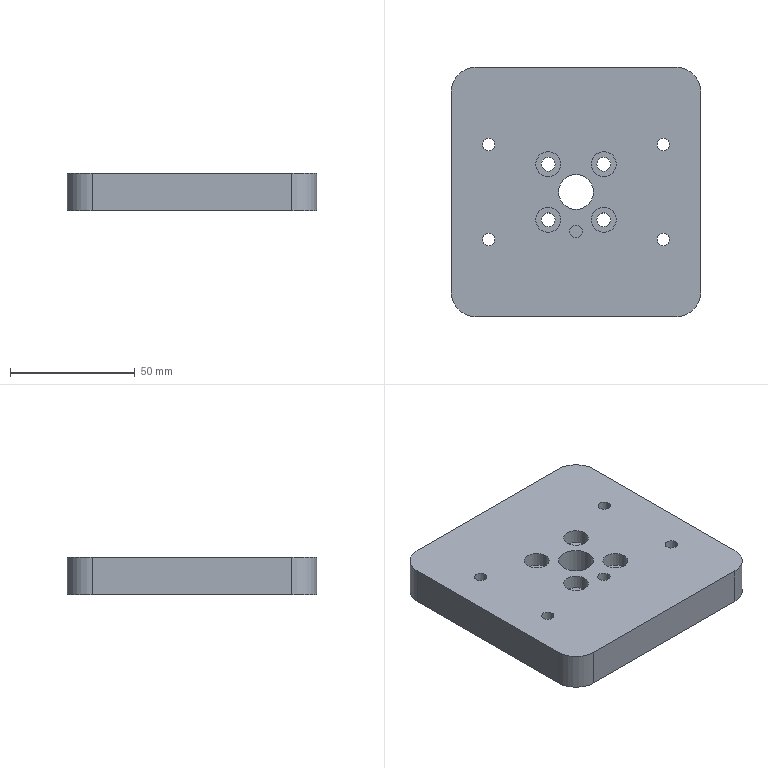NC program | NX | posted with a generic post | part box 100 x 100 x 15 mm
Lines 25 to 851 of 2072:
(ZLEVEL_PROFILE , TOOL : D10)
N48 T10 M6
N50 G54
N52 G17 G0 G90 X-53.748 Y-46.229 S9500 M3
N54 G43 Z30. H10
N56 Z1.5
N58 G94 G1 X-54.028 Y-45.669 Z1.467 F1000.
N60 X-54.754 Y-43.354 Z1.34
N62 X-55.1 Y-40.952 Z1.213
N64 Y-40. Z1.163
N66 Y0. Z-0.933
N68 Y40. F3500.
N70 G2 X-40. Y55.1 R15.1
N72 G1 X40.
N74 G2 X55.1 Y40. R15.1
N76 G1 Y-40.
N78 G2 X40. Y-55.1 R15.1
N80 G1 X-40.
N82 G2 X-55.1 Y-40. R15.1
N84 G1 Y0.
N86 Y40. Z-1.023
N88 X-55.072 Y40.912 Z-1.025
N90 X-54.99 Y41.82 Z-1.027
N92 X-54.853 Y42.722 Z-1.029
N94 X-54.661 Y43.614 Z-1.032
N96 X-54.416 Y44.492 Z-1.034
N98 X-54.119 Y45.355 Z-1.036
N100 X-53.77 Y46.197 Z-1.038
N102 X-53.37 Y47.017 Z-1.04
N104 X-52.922 Y47.812 Z-1.042
N106 X-52.427 Y48.578 Z-1.044
N108 X-51.886 Y49.312 Z-1.046
N110 X-51.303 Y50.013 Z-1.048
N112 X-50.677 Y50.677 Z-1.05
N114 X-50.013 Y51.303 Z-1.052
N116 X-49.312 Y51.886 Z-1.054
N118 X-48.578 Y52.427 Z-1.056
N120 X-47.812 Y52.922 Z-1.058
N122 X-47.017 Y53.37 Z-1.06
N124 X-46.197 Y53.77 Z-1.062
N126 X-45.355 Y54.119 Z-1.064
N128 X-44.492 Y54.416 Z-1.066
N130 X-43.614 Y54.661 Z-1.068
N132 X-42.722 Y54.853 Z-1.071
N134 X-41.82 Y54.99 Z-1.073
N136 X-40.912 Y55.072 Z-1.075
N138 X-40. Y55.1 Z-1.077
N140 X40. Z-1.257
N142 X40.912 Y55.072 Z-1.259
N144 X41.82 Y54.99 Z-1.261
N146 X42.722 Y54.853 Z-1.263
N148 X43.614 Y54.661 Z-1.265
N150 X44.492 Y54.416 Z-1.267
N152 X45.355 Y54.119 Z-1.269
N154 X46.197 Y53.77 Z-1.271
N156 X47.017 Y53.37 Z-1.273
N158 X47.812 Y52.922 Z-1.275
N160 X48.578 Y52.427 Z-1.277
N162 X49.312 Y51.886 Z-1.279
N164 X50.013 Y51.303 Z-1.281
N166 X50.677 Y50.677 Z-1.283
N168 X51.303 Y50.013 Z-1.285
N170 X51.886 Y49.312 Z-1.287
N172 X52.427 Y48.578 Z-1.289
N174 X52.922 Y47.812 Z-1.292
N176 X53.37 Y47.017 Z-1.294
N178 X53.77 Y46.197 Z-1.296
N180 X54.119 Y45.355 Z-1.298
N182 X54.416 Y44.492 Z-1.3
N184 X54.661 Y43.614 Z-1.302
N186 X54.853 Y42.722 Z-1.304
N188 X54.99 Y41.82 Z-1.306
N190 X55.072 Y40.912 Z-1.308
N192 X55.1 Y40. Z-1.31
N194 Y-40. Z-1.49
N196 X55.072 Y-40.912 Z-1.492
N198 X54.99 Y-41.82 Z-1.494
N200 X54.853 Y-42.722 Z-1.496
N202 X54.661 Y-43.614 Z-1.498
N204 X54.416 Y-44.492 Z-1.5
N206 X54.119 Y-45.355 Z-1.502
N208 X53.77 Y-46.197 Z-1.504
N210 X53.37 Y-47.017 Z-1.506
N212 X52.922 Y-47.812 Z-1.508
N214 X52.427 Y-48.578 Z-1.511
N216 X51.886 Y-49.312 Z-1.513
N218 X51.303 Y-50.013 Z-1.515
N220 X50.677 Y-50.677 Z-1.517
N222 X50.013 Y-51.303 Z-1.519
N224 X49.312 Y-51.886 Z-1.521
N226 X48.578 Y-52.427 Z-1.523
N228 X47.812 Y-52.922 Z-1.525
N230 X47.017 Y-53.37 Z-1.527
N232 X46.197 Y-53.77 Z-1.529
N234 X45.355 Y-54.119 Z-1.531
N236 X44.492 Y-54.416 Z-1.533
N238 X43.614 Y-54.661 Z-1.535
N240 X42.722 Y-54.853 Z-1.537
N242 X41.82 Y-54.99 Z-1.539
N244 X40.912 Y-55.072 Z-1.541
N246 X40. Y-55.1 Z-1.543
N248 X-40. Z-1.723
N250 X-40.912 Y-55.072 Z-1.725
N252 X-41.82 Y-54.99 Z-1.727
N254 X-42.722 Y-54.853 Z-1.729
N256 X-43.614 Y-54.661 Z-1.732
N258 X-44.492 Y-54.416 Z-1.734
N260 X-45.355 Y-54.119 Z-1.736
N262 X-46.197 Y-53.77 Z-1.738
N264 X-47.017 Y-53.37 Z-1.74
N266 X-47.812 Y-52.922 Z-1.742
N268 X-48.578 Y-52.427 Z-1.744
N270 X-49.312 Y-51.886 Z-1.746
N272 X-50.013 Y-51.303 Z-1.748
N274 X-50.677 Y-50.677 Z-1.75
N276 X-51.303 Y-50.013 Z-1.752
N278 X-51.886 Y-49.312 Z-1.754
N280 X-52.427 Y-48.578 Z-1.756
N282 X-52.922 Y-47.812 Z-1.758
N284 X-53.37 Y-47.017 Z-1.76
N286 X-53.77 Y-46.197 Z-1.762
N288 X-54.119 Y-45.355 Z-1.764
N290 X-54.416 Y-44.492 Z-1.766
N292 X-54.661 Y-43.614 Z-1.768
N294 X-54.853 Y-42.722 Z-1.771
N296 X-54.99 Y-41.82 Z-1.773
N298 X-55.072 Y-40.912 Z-1.775
N300 X-55.1 Y-40. Z-1.777
N302 Y0. Z-1.867
N304 Y40. Z-1.957
N306 X-55.072 Y40.912 Z-1.959
N308 X-54.99 Y41.82 Z-1.961
N310 X-54.853 Y42.722 Z-1.963
N312 X-54.661 Y43.614 Z-1.965
N314 X-54.416 Y44.492 Z-1.967
N316 X-54.119 Y45.355 Z-1.969
N318 X-53.77 Y46.197 Z-1.971
N320 X-53.37 Y47.017 Z-1.973
N322 X-52.922 Y47.812 Z-1.975
N324 X-52.427 Y48.578 Z-1.977
N326 X-51.886 Y49.312 Z-1.979
N328 X-51.303 Y50.013 Z-1.981
N330 X-50.677 Y50.677 Z-1.983
N332 X-50.013 Y51.303 Z-1.985
N334 X-49.312 Y51.886 Z-1.987
N336 X-48.578 Y52.427 Z-1.989
N338 X-47.812 Y52.922 Z-1.992
N340 X-47.017 Y53.37 Z-1.994
N342 X-46.197 Y53.77 Z-1.996
N344 X-45.355 Y54.119 Z-1.998
N346 X-44.492 Y54.416 Z-2.
N348 X-43.614 Y54.661 Z-2.002
N350 X-42.722 Y54.853 Z-2.004
N352 X-41.82 Y54.99 Z-2.006
N354 X-40.912 Y55.072 Z-2.008
N356 X-40. Y55.1 Z-2.01
N358 X40. Z-2.19
N360 X40.912 Y55.072 Z-2.192
N362 X41.82 Y54.99 Z-2.194
N364 X42.722 Y54.853 Z-2.196
N366 X43.614 Y54.661 Z-2.198
N368 X44.492 Y54.416 Z-2.2
N370 X45.355 Y54.119 Z-2.202
N372 X46.197 Y53.77 Z-2.204
N374 X47.017 Y53.37 Z-2.206
N376 X47.812 Y52.922 Z-2.208
N378 X48.578 Y52.427 Z-2.211
N380 X49.312 Y51.886 Z-2.213
N382 X50.013 Y51.303 Z-2.215
N384 X50.677 Y50.677 Z-2.217
N386 X51.303 Y50.013 Z-2.219
N388 X51.886 Y49.312 Z-2.221
N390 X52.427 Y48.578 Z-2.223
N392 X52.922 Y47.812 Z-2.225
N394 X53.37 Y47.017 Z-2.227
N396 X53.77 Y46.197 Z-2.229
N398 X54.119 Y45.355 Z-2.231
N400 X54.416 Y44.492 Z-2.233
N402 X54.661 Y43.614 Z-2.235
N404 X54.853 Y42.722 Z-2.237
N406 X54.99 Y41.82 Z-2.239
N408 X55.072 Y40.912 Z-2.241
N410 X55.1 Y40. Z-2.243
N412 Y-40. Z-2.423
N414 X55.072 Y-40.912 Z-2.425
N416 X54.99 Y-41.82 Z-2.427
N418 X54.853 Y-42.722 Z-2.429
N420 X54.661 Y-43.614 Z-2.432
N422 X54.416 Y-44.492 Z-2.434
N424 X54.119 Y-45.355 Z-2.436
N426 X53.77 Y-46.197 Z-2.438
N428 X53.37 Y-47.017 Z-2.44
N430 X52.922 Y-47.812 Z-2.442
N432 X52.427 Y-48.578 Z-2.444
N434 X51.886 Y-49.312 Z-2.446
N436 X51.303 Y-50.013 Z-2.448
N438 X50.677 Y-50.677 Z-2.45
N440 X50.013 Y-51.303 Z-2.452
N442 X49.312 Y-51.886 Z-2.454
N444 X48.578 Y-52.427 Z-2.456
N446 X47.812 Y-52.922 Z-2.458
N448 X47.017 Y-53.37 Z-2.46
N450 X46.197 Y-53.77 Z-2.462
N452 X45.355 Y-54.119 Z-2.464
N454 X44.492 Y-54.416 Z-2.466
N456 X43.614 Y-54.661 Z-2.468
N458 X42.722 Y-54.853 Z-2.471
N460 X41.82 Y-54.99 Z-2.473
N462 X40.912 Y-55.072 Z-2.475
N464 X40. Y-55.1 Z-2.477
N466 X-40. Z-2.657
N468 X-40.912 Y-55.072 Z-2.659
N470 X-41.82 Y-54.99 Z-2.661
N472 X-42.722 Y-54.853 Z-2.663
N474 X-43.614 Y-54.661 Z-2.665
N476 X-44.492 Y-54.416 Z-2.667
N478 X-45.355 Y-54.119 Z-2.669
N480 X-46.197 Y-53.77 Z-2.671
N482 X-47.017 Y-53.37 Z-2.673
N484 X-47.812 Y-52.922 Z-2.675
N486 X-48.578 Y-52.427 Z-2.677
N488 X-49.312 Y-51.886 Z-2.679
N490 X-50.013 Y-51.303 Z-2.681
N492 X-50.677 Y-50.677 Z-2.683
N494 X-51.303 Y-50.013 Z-2.685
N496 X-51.886 Y-49.312 Z-2.687
N498 X-52.427 Y-48.578 Z-2.689
N500 X-52.922 Y-47.812 Z-2.692
N502 X-53.37 Y-47.017 Z-2.694
N504 X-53.77 Y-46.197 Z-2.696
N506 X-54.119 Y-45.355 Z-2.698
N508 X-54.416 Y-44.492 Z-2.7
N510 X-54.661 Y-43.614 Z-2.702
N512 X-54.853 Y-42.722 Z-2.704
N514 X-54.99 Y-41.82 Z-2.706
N516 X-55.072 Y-40.912 Z-2.708
N518 X-55.1 Y-40. Z-2.71
N520 Y0. Z-2.8
N522 Y40. Z-2.89
N524 X-55.072 Y40.912 Z-2.892
N526 X-54.99 Y41.82 Z-2.894
N528 X-54.853 Y42.722 Z-2.896
N530 X-54.661 Y43.614 Z-2.898
N532 X-54.416 Y44.492 Z-2.9
N534 X-54.119 Y45.355 Z-2.902
N536 X-53.77 Y46.197 Z-2.904
N538 X-53.37 Y47.017 Z-2.906
N540 X-52.922 Y47.812 Z-2.908
N542 X-52.427 Y48.578 Z-2.911
N544 X-51.886 Y49.312 Z-2.913
N546 X-51.303 Y50.013 Z-2.915
N548 X-50.677 Y50.677 Z-2.917
N550 X-50.013 Y51.303 Z-2.919
N552 X-49.312 Y51.886 Z-2.921
N554 X-48.578 Y52.427 Z-2.923
N556 X-47.812 Y52.922 Z-2.925
N558 X-47.017 Y53.37 Z-2.927
N560 X-46.197 Y53.77 Z-2.929
N562 X-45.355 Y54.119 Z-2.931
N564 X-44.492 Y54.416 Z-2.933
N566 X-43.614 Y54.661 Z-2.935
N568 X-42.722 Y54.853 Z-2.937
N570 X-41.82 Y54.99 Z-2.939
N572 X-40.912 Y55.072 Z-2.941
N574 X-40. Y55.1 Z-2.943
N576 X40. Z-3.123
N578 X40.912 Y55.072 Z-3.125
N580 X41.82 Y54.99 Z-3.127
N582 X42.722 Y54.853 Z-3.129
N584 X43.614 Y54.661 Z-3.132
N586 X44.492 Y54.416 Z-3.134
N588 X45.355 Y54.119 Z-3.136
N590 X46.197 Y53.77 Z-3.138
N592 X47.017 Y53.37 Z-3.14
N594 X47.812 Y52.922 Z-3.142
N596 X48.578 Y52.427 Z-3.144
N598 X49.312 Y51.886 Z-3.146
N600 X50.013 Y51.303 Z-3.148
N602 X50.677 Y50.677 Z-3.15
N604 X51.303 Y50.013 Z-3.152
N606 X51.886 Y49.312 Z-3.154
N608 X52.427 Y48.578 Z-3.156
N610 X52.922 Y47.812 Z-3.158
N612 X53.37 Y47.017 Z-3.16
N614 X53.77 Y46.197 Z-3.162
N616 X54.119 Y45.355 Z-3.164
N618 X54.416 Y44.492 Z-3.166
N620 X54.661 Y43.614 Z-3.168
N622 X54.853 Y42.722 Z-3.171
N624 X54.99 Y41.82 Z-3.173
N626 X55.072 Y40.912 Z-3.175
N628 X55.1 Y40. Z-3.177
N630 Y-40. Z-3.357
N632 X55.072 Y-40.912 Z-3.359
N634 X54.99 Y-41.82 Z-3.361
N636 X54.853 Y-42.722 Z-3.363
N638 X54.661 Y-43.614 Z-3.365
N640 X54.416 Y-44.492 Z-3.367
N642 X54.119 Y-45.355 Z-3.369
N644 X53.77 Y-46.197 Z-3.371
N646 X53.37 Y-47.017 Z-3.373
N648 X52.922 Y-47.812 Z-3.375
N650 X52.427 Y-48.578 Z-3.377
N652 X51.886 Y-49.312 Z-3.379
N654 X51.303 Y-50.013 Z-3.381
N656 X50.677 Y-50.677 Z-3.383
N658 X50.013 Y-51.303 Z-3.385
N660 X49.312 Y-51.886 Z-3.387
N662 X48.578 Y-52.427 Z-3.389
N664 X47.812 Y-52.922 Z-3.392
N666 X47.017 Y-53.37 Z-3.394
N668 X46.197 Y-53.77 Z-3.396
N670 X45.355 Y-54.119 Z-3.398
N672 X44.492 Y-54.416 Z-3.4
N674 X43.614 Y-54.661 Z-3.402
N676 X42.722 Y-54.853 Z-3.404
N678 X41.82 Y-54.99 Z-3.406
N680 X40.912 Y-55.072 Z-3.408
N682 X40. Y-55.1 Z-3.41
N684 X-40. Z-3.59
N686 X-40.912 Y-55.072 Z-3.592
N688 X-41.82 Y-54.99 Z-3.594
N690 X-42.722 Y-54.853 Z-3.596
N692 X-43.614 Y-54.661 Z-3.598
N694 X-44.492 Y-54.416 Z-3.6
N696 X-45.355 Y-54.119 Z-3.602
N698 X-46.197 Y-53.77 Z-3.604
N700 X-47.017 Y-53.37 Z-3.606
N702 X-47.812 Y-52.922 Z-3.608
N704 X-48.578 Y-52.427 Z-3.611
N706 X-49.312 Y-51.886 Z-3.613
N708 X-50.013 Y-51.303 Z-3.615
N710 X-50.677 Y-50.677 Z-3.617
N712 X-51.303 Y-50.013 Z-3.619
N714 X-51.886 Y-49.312 Z-3.621
N716 X-52.427 Y-48.578 Z-3.623
N718 X-52.922 Y-47.812 Z-3.625
N720 X-53.37 Y-47.017 Z-3.627
N722 X-53.77 Y-46.197 Z-3.629
N724 X-54.119 Y-45.355 Z-3.631
N726 X-54.416 Y-44.492 Z-3.633
N728 X-54.661 Y-43.614 Z-3.635
N730 X-54.853 Y-42.722 Z-3.637
N732 X-54.99 Y-41.82 Z-3.639
N734 X-55.072 Y-40.912 Z-3.641
N736 X-55.1 Y-40. Z-3.643
N738 Y0. Z-3.733
N740 Y40. Z-3.823
N742 X-55.072 Y40.912 Z-3.825
N744 X-54.99 Y41.82 Z-3.827
N746 X-54.853 Y42.722 Z-3.829
N748 X-54.661 Y43.614 Z-3.832
N750 X-54.416 Y44.492 Z-3.834
N752 X-54.119 Y45.355 Z-3.836
N754 X-53.77 Y46.197 Z-3.838
N756 X-53.37 Y47.017 Z-3.84
N758 X-52.922 Y47.812 Z-3.842
N760 X-52.427 Y48.578 Z-3.844
N762 X-51.886 Y49.312 Z-3.846
N764 X-51.303 Y50.013 Z-3.848
N766 X-50.677 Y50.677 Z-3.85
N768 X-50.013 Y51.303 Z-3.852
N770 X-49.312 Y51.886 Z-3.854
N772 X-48.578 Y52.427 Z-3.856
N774 X-47.812 Y52.922 Z-3.858
N776 X-47.017 Y53.37 Z-3.86
N778 X-46.197 Y53.77 Z-3.862
N780 X-45.355 Y54.119 Z-3.864
N782 X-44.492 Y54.416 Z-3.866
N784 X-43.614 Y54.661 Z-3.868
N786 X-42.722 Y54.853 Z-3.871
N788 X-41.82 Y54.99 Z-3.873
N790 X-40.912 Y55.072 Z-3.875
N792 X-40. Y55.1 Z-3.877
N794 X40. Z-4.057
N796 X40.912 Y55.072 Z-4.059
N798 X41.82 Y54.99 Z-4.061
N800 X42.722 Y54.853 Z-4.063
N802 X43.614 Y54.661 Z-4.065
N804 X44.492 Y54.416 Z-4.067
N806 X45.355 Y54.119 Z-4.069
N808 X46.197 Y53.77 Z-4.071
N810 X47.017 Y53.37 Z-4.073
N812 X47.812 Y52.922 Z-4.075
N814 X48.578 Y52.427 Z-4.077
N816 X49.312 Y51.886 Z-4.079
N818 X50.013 Y51.303 Z-4.081
N820 X50.677 Y50.677 Z-4.083
N822 X51.303 Y50.013 Z-4.085
N824 X51.886 Y49.312 Z-4.087
N826 X52.427 Y48.578 Z-4.089
N828 X52.922 Y47.812 Z-4.092
N830 X53.37 Y47.017 Z-4.094
N832 X53.77 Y46.197 Z-4.096
N834 X54.119 Y45.355 Z-4.098
N836 X54.416 Y44.492 Z-4.1
N838 X54.661 Y43.614 Z-4.102
N840 X54.853 Y42.722 Z-4.104
N842 X54.99 Y41.82 Z-4.106
N844 X55.072 Y40.912 Z-4.108
N846 X55.1 Y40. Z-4.11
N848 Y-40. Z-4.29
N850 X55.072 Y-40.912 Z-4.292
N852 X54.99 Y-41.82 Z-4.294
N854 X54.853 Y-42.722 Z-4.296
N856 X54.661 Y-43.614 Z-4.298
N858 X54.416 Y-44.492 Z-4.3
N860 X54.119 Y-45.355 Z-4.302
N862 X53.77 Y-46.197 Z-4.304
N864 X53.37 Y-47.017 Z-4.306
N866 X52.922 Y-47.812 Z-4.308
N868 X52.427 Y-48.578 Z-4.311
N870 X51.886 Y-49.312 Z-4.313
N872 X51.303 Y-50.013 Z-4.315
N874 X50.677 Y-50.677 Z-4.317
N876 X50.013 Y-51.303 Z-4.319
N878 X49.312 Y-51.886 Z-4.321
N880 X48.578 Y-52.427 Z-4.323
N882 X47.812 Y-52.922 Z-4.325
N884 X47.017 Y-53.37 Z-4.327
N886 X46.197 Y-53.77 Z-4.329
N888 X45.355 Y-54.119 Z-4.331
N890 X44.492 Y-54.416 Z-4.333
N892 X43.614 Y-54.661 Z-4.335
N894 X42.722 Y-54.853 Z-4.337
N896 X41.82 Y-54.99 Z-4.339
N898 X40.912 Y-55.072 Z-4.341
N900 X40. Y-55.1 Z-4.343
N902 X-40. Z-4.523
N904 X-40.912 Y-55.072 Z-4.525
N906 X-41.82 Y-54.99 Z-4.527
N908 X-42.722 Y-54.853 Z-4.529
N910 X-43.614 Y-54.661 Z-4.532
N912 X-44.492 Y-54.416 Z-4.534
N914 X-45.355 Y-54.119 Z-4.536
N916 X-46.197 Y-53.77 Z-4.538
N918 X-47.017 Y-53.37 Z-4.54
N920 X-47.812 Y-52.922 Z-4.542
N922 X-48.578 Y-52.427 Z-4.544
N924 X-49.312 Y-51.886 Z-4.546
N926 X-50.013 Y-51.303 Z-4.548
N928 X-50.677 Y-50.677 Z-4.55
N930 X-51.303 Y-50.013 Z-4.552
N932 X-51.886 Y-49.312 Z-4.554
N934 X-52.427 Y-48.578 Z-4.556
N936 X-52.922 Y-47.812 Z-4.558
N938 X-53.37 Y-47.017 Z-4.56
N940 X-53.77 Y-46.197 Z-4.562
N942 X-54.119 Y-45.355 Z-4.564
N944 X-54.416 Y-44.492 Z-4.566
N946 X-54.661 Y-43.614 Z-4.568
N948 X-54.853 Y-42.722 Z-4.571
N950 X-54.99 Y-41.82 Z-4.573
N952 X-55.072 Y-40.912 Z-4.575
N954 X-55.1 Y-40. Z-4.577
N956 Y0. Z-4.667
N958 Y40. Z-4.757
N960 X-55.072 Y40.912 Z-4.759
N962 X-54.99 Y41.82 Z-4.761
N964 X-54.853 Y42.722 Z-4.763
N966 X-54.661 Y43.614 Z-4.765
N968 X-54.416 Y44.492 Z-4.767
N970 X-54.119 Y45.355 Z-4.769
N972 X-53.77 Y46.197 Z-4.771
N974 X-53.37 Y47.017 Z-4.773
N976 X-52.922 Y47.812 Z-4.775
N978 X-52.427 Y48.578 Z-4.777
N980 X-51.886 Y49.312 Z-4.779
N982 X-51.303 Y50.013 Z-4.781
N984 X-50.677 Y50.677 Z-4.783
N986 X-50.013 Y51.303 Z-4.785
N988 X-49.312 Y51.886 Z-4.787
N990 X-48.578 Y52.427 Z-4.789
N992 X-47.812 Y52.922 Z-4.792
N994 X-47.017 Y53.37 Z-4.794
N996 X-46.197 Y53.77 Z-4.796
N998 X-45.355 Y54.119 Z-4.798
N1000 X-44.492 Y54.416 Z-4.8
N1002 X-43.614 Y54.661 Z-4.802
N1004 X-42.722 Y54.853 Z-4.804
N1006 X-41.82 Y54.99 Z-4.806
N1008 X-40.912 Y55.072 Z-4.808
N1010 X-40. Y55.1 Z-4.81
N1012 X40. Z-4.99
N1014 X40.912 Y55.072 Z-4.992
N1016 X41.82 Y54.99 Z-4.994
N1018 X42.722 Y54.853 Z-4.996
N1020 X43.614 Y54.661 Z-4.998
N1022 X44.492 Y54.416 Z-5.
N1024 X45.355 Y54.119 Z-5.002
N1026 X46.197 Y53.77 Z-5.004
N1028 X47.017 Y53.37 Z-5.006
N1030 X47.812 Y52.922 Z-5.008
N1032 X48.578 Y52.427 Z-5.011
N1034 X49.312 Y51.886 Z-5.013
N1036 X50.013 Y51.303 Z-5.015
N1038 X50.677 Y50.677 Z-5.017
N1040 X51.303 Y50.013 Z-5.019
N1042 X51.886 Y49.312 Z-5.021
N1044 X52.427 Y48.578 Z-5.023
N1046 X52.922 Y47.812 Z-5.025
N1048 X53.37 Y47.017 Z-5.027
N1050 X53.77 Y46.197 Z-5.029
N1052 X54.119 Y45.355 Z-5.031
N1054 X54.416 Y44.492 Z-5.033
N1056 X54.661 Y43.614 Z-5.035
N1058 X54.853 Y42.722 Z-5.037
N1060 X54.99 Y41.82 Z-5.039
N1062 X55.072 Y40.912 Z-5.041
N1064 X55.1 Y40. Z-5.043
N1066 Y-40. Z-5.223
N1068 X55.072 Y-40.912 Z-5.225
N1070 X54.99 Y-41.82 Z-5.227
N1072 X54.853 Y-42.722 Z-5.229
N1074 X54.661 Y-43.614 Z-5.232
N1076 X54.416 Y-44.492 Z-5.234
N1078 X54.119 Y-45.355 Z-5.236
N1080 X53.77 Y-46.197 Z-5.238
N1082 X53.37 Y-47.017 Z-5.24
N1084 X52.922 Y-47.812 Z-5.242
N1086 X52.427 Y-48.578 Z-5.244
N1088 X51.886 Y-49.312 Z-5.246
N1090 X51.303 Y-50.013 Z-5.248
N1092 X50.677 Y-50.677 Z-5.25
N1094 X50.013 Y-51.303 Z-5.252
N1096 X49.312 Y-51.886 Z-5.254
N1098 X48.578 Y-52.427 Z-5.256
N1100 X47.812 Y-52.922 Z-5.258
N1102 X47.017 Y-53.37 Z-5.26
N1104 X46.197 Y-53.77 Z-5.262
N1106 X45.355 Y-54.119 Z-5.264
N1108 X44.492 Y-54.416 Z-5.266
N1110 X43.614 Y-54.661 Z-5.268
N1112 X42.722 Y-54.853 Z-5.271
N1114 X41.82 Y-54.99 Z-5.273
N1116 X40.912 Y-55.072 Z-5.275
N1118 X40. Y-55.1 Z-5.277
N1120 X-40. Z-5.457
N1122 X-40.912 Y-55.072 Z-5.459
N1124 X-41.82 Y-54.99 Z-5.461
N1126 X-42.722 Y-54.853 Z-5.463
N1128 X-43.614 Y-54.661 Z-5.465
N1130 X-44.492 Y-54.416 Z-5.467
N1132 X-45.355 Y-54.119 Z-5.469
N1134 X-46.197 Y-53.77 Z-5.471
N1136 X-47.017 Y-53.37 Z-5.473
N1138 X-47.812 Y-52.922 Z-5.475
N1140 X-48.578 Y-52.427 Z-5.477
N1142 X-49.312 Y-51.886 Z-5.479
N1144 X-50.013 Y-51.303 Z-5.481
N1146 X-50.677 Y-50.677 Z-5.483
N1148 X-51.303 Y-50.013 Z-5.485
N1150 X-51.886 Y-49.312 Z-5.487
N1152 X-52.427 Y-48.578 Z-5.489
N1154 X-52.922 Y-47.812 Z-5.492
N1156 X-53.37 Y-47.017 Z-5.494
N1158 X-53.77 Y-46.197 Z-5.496
N1160 X-54.119 Y-45.355 Z-5.498
N1162 X-54.416 Y-44.492 Z-5.5
N1164 X-54.661 Y-43.614 Z-5.502
N1166 X-54.853 Y-42.722 Z-5.504
N1168 X-54.99 Y-41.82 Z-5.506
N1170 X-55.072 Y-40.912 Z-5.508
N1172 X-55.1 Y-40. Z-5.51
N1174 Y0. Z-5.6
N1176 Y40. Z-5.677
N1178 X-55.072 Y40.912 Z-5.679
N1180 X-54.99 Y41.82 Z-5.681
N1182 X-54.853 Y42.722 Z-5.682
N1184 X-54.661 Y43.614 Z-5.684
N1186 X-54.416 Y44.492 Z-5.686
N1188 X-54.119 Y45.355 Z-5.688
N1190 X-53.77 Y46.197 Z-5.689
N1192 X-53.37 Y47.017 Z-5.691
N1194 X-52.922 Y47.812 Z-5.693
N1196 X-52.427 Y48.578 Z-5.695
N1198 X-51.886 Y49.312 Z-5.696
N1200 X-51.303 Y50.013 Z-5.698
N1202 X-50.677 Y50.677 Z-5.7
N1204 X-50.013 Y51.303 Z-5.702
N1206 X-49.312 Y51.886 Z-5.704
N1208 X-48.578 Y52.427 Z-5.705
N1210 X-47.812 Y52.922 Z-5.707
N1212 X-47.017 Y53.37 Z-5.709
N1214 X-46.197 Y53.77 Z-5.711
N1216 X-45.355 Y54.119 Z-5.712
N1218 X-44.492 Y54.416 Z-5.714
N1220 X-43.614 Y54.661 Z-5.716
N1222 X-42.722 Y54.853 Z-5.718
N1224 X-41.82 Y54.99 Z-5.719
N1226 X-40.912 Y55.072 Z-5.721
N1228 X-40. Y55.1 Z-5.723
N1230 X40. Z-5.877
N1232 X40.912 Y55.072 Z-5.879
N1234 X41.82 Y54.99 Z-5.881
N1236 X42.722 Y54.853 Z-5.882
N1238 X43.614 Y54.661 Z-5.884
N1240 X44.492 Y54.416 Z-5.886
N1242 X45.355 Y54.119 Z-5.888
N1244 X46.197 Y53.77 Z-5.889
N1246 X47.017 Y53.37 Z-5.891
N1248 X47.812 Y52.922 Z-5.893
N1250 X48.578 Y52.427 Z-5.895
N1252 X49.312 Y51.886 Z-5.896
N1254 X50.013 Y51.303 Z-5.898
N1256 X50.677 Y50.677 Z-5.9
N1258 X51.303 Y50.013 Z-5.902
N1260 X51.886 Y49.312 Z-5.904
N1262 X52.427 Y48.578 Z-5.905
N1264 X52.922 Y47.812 Z-5.907
N1266 X53.37 Y47.017 Z-5.909
N1268 X53.77 Y46.197 Z-5.911
N1270 X54.119 Y45.355 Z-5.912
N1272 X54.416 Y44.492 Z-5.914
N1274 X54.661 Y43.614 Z-5.916
N1276 X54.853 Y42.722 Z-5.918
N1278 X54.99 Y41.82 Z-5.919
N1280 X55.072 Y40.912 Z-5.921
N1282 X55.1 Y40. Z-5.923
N1284 Y-40. Z-6.077
N1286 X55.072 Y-40.912 Z-6.079
N1288 X54.99 Y-41.82 Z-6.081
N1290 X54.853 Y-42.722 Z-6.082
N1292 X54.661 Y-43.614 Z-6.084
N1294 X54.416 Y-44.492 Z-6.086
N1296 X54.119 Y-45.355 Z-6.088
N1298 X53.77 Y-46.197 Z-6.089
N1300 X53.37 Y-47.017 Z-6.091
N1302 X52.922 Y-47.812 Z-6.093
N1304 X52.427 Y-48.578 Z-6.095
N1306 X51.886 Y-49.312 Z-6.096
N1308 X51.303 Y-50.013 Z-6.098
N1310 X50.677 Y-50.677 Z-6.1
N1312 X50.013 Y-51.303 Z-6.102
N1314 X49.312 Y-51.886 Z-6.104
N1316 X48.578 Y-52.427 Z-6.105
N1318 X47.812 Y-52.922 Z-6.107
N1320 X47.017 Y-53.37 Z-6.109
N1322 X46.197 Y-53.77 Z-6.111
N1324 X45.355 Y-54.119 Z-6.112
N1326 X44.492 Y-54.416 Z-6.114
N1328 X43.614 Y-54.661 Z-6.116
N1330 X42.722 Y-54.853 Z-6.118
N1332 X41.82 Y-54.99 Z-6.119
N1334 X40.912 Y-55.072 Z-6.121
N1336 X40. Y-55.1 Z-6.123
N1338 X-40. Z-6.277
N1340 X-40.912 Y-55.072 Z-6.279
N1342 X-41.82 Y-54.99 Z-6.281
N1344 X-42.722 Y-54.853 Z-6.282
N1346 X-43.614 Y-54.661 Z-6.284
N1348 X-44.492 Y-54.416 Z-6.286
N1350 X-45.355 Y-54.119 Z-6.288
N1352 X-46.197 Y-53.77 Z-6.289
N1354 X-47.017 Y-53.37 Z-6.291
N1356 X-47.812 Y-52.922 Z-6.293
N1358 X-48.578 Y-52.427 Z-6.295
N1360 X-49.312 Y-51.886 Z-6.296
N1362 X-50.013 Y-51.303 Z-6.298
N1364 X-50.677 Y-50.677 Z-6.3
N1366 X-51.303 Y-50.013 Z-6.302
N1368 X-51.886 Y-49.312 Z-6.304
N1370 X-52.427 Y-48.578 Z-6.305
N1372 X-52.922 Y-47.812 Z-6.307
N1374 X-53.37 Y-47.017 Z-6.309
N1376 X-53.77 Y-46.197 Z-6.311
N1378 X-54.119 Y-45.355 Z-6.312
N1380 X-54.416 Y-44.492 Z-6.314
N1382 X-54.661 Y-43.614 Z-6.316
N1384 X-54.853 Y-42.722 Z-6.318
N1386 X-54.99 Y-41.82 Z-6.319
N1388 X-55.072 Y-40.912 Z-6.321
N1390 X-55.1 Y-40. Z-6.323
N1392 Y0. Z-6.4
N1394 Y40. Z-6.492
N1396 X-55.072 Y40.912 Z-6.494
N1398 X-54.99 Y41.82 Z-6.496
N1400 X-54.853 Y42.722 Z-6.498
N1402 X-54.661 Y43.614 Z-6.501
N1404 X-54.416 Y44.492 Z-6.503
N1406 X-54.119 Y45.355 Z-6.505
N1408 X-53.77 Y46.197 Z-6.507
N1410 X-53.37 Y47.017 Z-6.509
N1412 X-52.922 Y47.812 Z-6.511
N1414 X-52.427 Y48.578 Z-6.513
N1416 X-51.886 Y49.312 Z-6.515
N1418 X-51.303 Y50.013 Z-6.517
N1420 X-50.677 Y50.677 Z-6.519
N1422 X-50.013 Y51.303 Z-6.522
N1424 X-49.312 Y51.886 Z-6.524
N1426 X-48.578 Y52.427 Z-6.526
N1428 X-47.812 Y52.922 Z-6.528
N1430 X-47.017 Y53.37 Z-6.53
N1432 X-46.197 Y53.77 Z-6.532
N1434 X-45.355 Y54.119 Z-6.534
N1436 X-44.492 Y54.416 Z-6.536
N1438 X-43.614 Y54.661 Z-6.538
N1440 X-42.722 Y54.853 Z-6.54
N1442 X-41.82 Y54.99 Z-6.543
N1444 X-40.912 Y55.072 Z-6.545
N1446 X-40. Y55.1 Z-6.547
N1448 X40. Z-6.731
N1450 X40.912 Y55.072 Z-6.733
N1452 X41.82 Y54.99 Z-6.735
N1454 X42.722 Y54.853 Z-6.737
N1456 X43.614 Y54.661 Z-6.739
N1458 X44.492 Y54.416 Z-6.742
N1460 X45.355 Y54.119 Z-6.744
N1462 X46.197 Y53.77 Z-6.746
N1464 X47.017 Y53.37 Z-6.748
N1466 X47.812 Y52.922 Z-6.75
N1468 X48.578 Y52.427 Z-6.752
N1470 X49.312 Y51.886 Z-6.754
N1472 X50.013 Y51.303 Z-6.756
N1474 X50.677 Y50.677 Z-6.758
N1476 X51.303 Y50.013 Z-6.76
N1478 X51.886 Y49.312 Z-6.763
N1480 X52.427 Y48.578 Z-6.765
N1482 X52.922 Y47.812 Z-6.767
N1484 X53.37 Y47.017 Z-6.769
N1486 X53.77 Y46.197 Z-6.771
N1488 X54.119 Y45.355 Z-6.773
N1490 X54.416 Y44.492 Z-6.775
N1492 X54.661 Y43.614 Z-6.777
N1494 X54.853 Y42.722 Z-6.779
N1496 X54.99 Y41.82 Z-6.781
N1498 X55.072 Y40.912 Z-6.784
N1500 X55.1 Y40. Z-6.786
N1502 Y-40. Z-6.97
N1504 X55.072 Y-40.912 Z-6.972
N1506 X54.99 Y-41.82 Z-6.974
N1508 X54.853 Y-42.722 Z-6.976
N1510 X54.661 Y-43.614 Z-6.978
N1512 X54.416 Y-44.492 Z-6.98
N1514 X54.119 Y-45.355 Z-6.983
N1516 X53.77 Y-46.197 Z-6.985
N1518 X53.37 Y-47.017 Z-6.987
N1520 X52.922 Y-47.812 Z-6.989
N1522 X52.427 Y-48.578 Z-6.991
N1524 X51.886 Y-49.312 Z-6.993
N1526 X51.303 Y-50.013 Z-6.995
N1528 X50.677 Y-50.677 Z-6.997
N1530 X50.013 Y-51.303 Z-6.999
N1532 X49.312 Y-51.886 Z-7.001
N1534 X48.578 Y-52.427 Z-7.004
N1536 X47.812 Y-52.922 Z-7.006
N1538 X47.017 Y-53.37 Z-7.008
N1540 X46.197 Y-53.77 Z-7.01
N1542 X45.355 Y-54.119 Z-7.012
N1544 X44.492 Y-54.416 Z-7.014
N1546 X43.614 Y-54.661 Z-7.016
N1548 X42.722 Y-54.853 Z-7.018
N1550 X41.82 Y-54.99 Z-7.02
N1552 X40.912 Y-55.072 Z-7.022
N1554 X40. Y-55.1 Z-7.025
N1556 X-40. Z-7.209
N1558 X-40.912 Y-55.072 Z-7.211
N1560 X-41.82 Y-54.99 Z-7.213
N1562 X-42.722 Y-54.853 Z-7.215
N1564 X-43.614 Y-54.661 Z-7.217
N1566 X-44.492 Y-54.416 Z-7.219
N1568 X-45.355 Y-54.119 Z-7.221
N1570 X-46.197 Y-53.77 Z-7.224
N1572 X-47.017 Y-53.37 Z-7.226
N1574 X-47.812 Y-52.922 Z-7.228
N1576 X-48.578 Y-52.427 Z-7.23
N1578 X-49.312 Y-51.886 Z-7.232
N1580 X-50.013 Y-51.303 Z-7.234
N1582 X-50.677 Y-50.677 Z-7.236
N1584 X-51.303 Y-50.013 Z-7.238
N1586 X-51.886 Y-49.312 Z-7.24
N1588 X-52.427 Y-48.578 Z-7.242
N1590 X-52.922 Y-47.812 Z-7.245
N1592 X-53.37 Y-47.017 Z-7.247
N1594 X-53.77 Y-46.197 Z-7.249
N1596 X-54.119 Y-45.355 Z-7.251
N1598 X-54.416 Y-44.492 Z-7.253
N1600 X-54.661 Y-43.614 Z-7.255
N1602 X-54.853 Y-42.722 Z-7.257
N1604 X-54.99 Y-41.82 Z-7.259
N1606 X-55.072 Y-40.912 Z-7.261
N1608 X-55.1 Y-40. Z-7.263
N1610 Y0. Z-7.356
N1612 Y40. Z-7.448
N1614 X-55.072 Y40.912 Z-7.45
N1616 X-54.99 Y41.82 Z-7.452
N1618 X-54.853 Y42.722 Z-7.454
N1620 X-54.661 Y43.614 Z-7.456
N1622 X-54.416 Y44.492 Z-7.458
N1624 X-54.119 Y45.355 Z-7.46
N1626 X-53.77 Y46.197 Z-7.462
N1628 X-53.37 Y47.017 Z-7.465
N1630 X-52.922 Y47.812 Z-7.467
N1632 X-52.427 Y48.578 Z-7.469
N1634 X-51.886 Y49.312 Z-7.471
N1636 X-51.303 Y50.013 Z-7.473
N1638 X-50.677 Y50.677 Z-7.475
N1640 X-50.013 Y51.303 Z-7.477
N1642 X-49.312 Y51.886 Z-7.479
N1644 X-48.578 Y52.427 Z-7.481
N1646 X-47.812 Y52.922 Z-7.483
N1648 X-47.017 Y53.37 Z-7.486
N1650 X-46.197 Y53.77 Z-7.488
N1652 X-45.355 Y54.119 Z-7.49
N1654 X-44.492 Y54.416 Z-7.492
N1656 X-43.614 Y54.661 Z-7.494
N1658 X-42.722 Y54.853 Z-7.496
N1660 X-41.82 Y54.99 Z-7.498
N1662 X-40.912 Y55.072 Z-7.5
N1664 X-40. Y55.1 Z-7.502
N1666 X40. Z-7.687
N1668 X40.912 Y55.072 Z-7.689
N1670 X41.82 Y54.99 Z-7.691
N1672 X42.722 Y54.853 Z-7.693
N1674 X43.614 Y54.661 Z-7.695
N1676 X44.492 Y54.416 Z-7.697
N1678 X45.355 Y54.119 Z-7.699
N1680 X46.197 Y53.77 Z-7.701
N1682 X47.017 Y53.37 Z-7.703
N1684 X47.812 Y52.922 Z-7.705
N1686 X48.578 Y52.427 Z-7.708
N1688 X49.312 Y51.886 Z-7.71
N1690 X50.013 Y51.303 Z-7.712
N1692 X50.677 Y50.677 Z-7.714
N1694 X51.303 Y50.013 Z-7.716